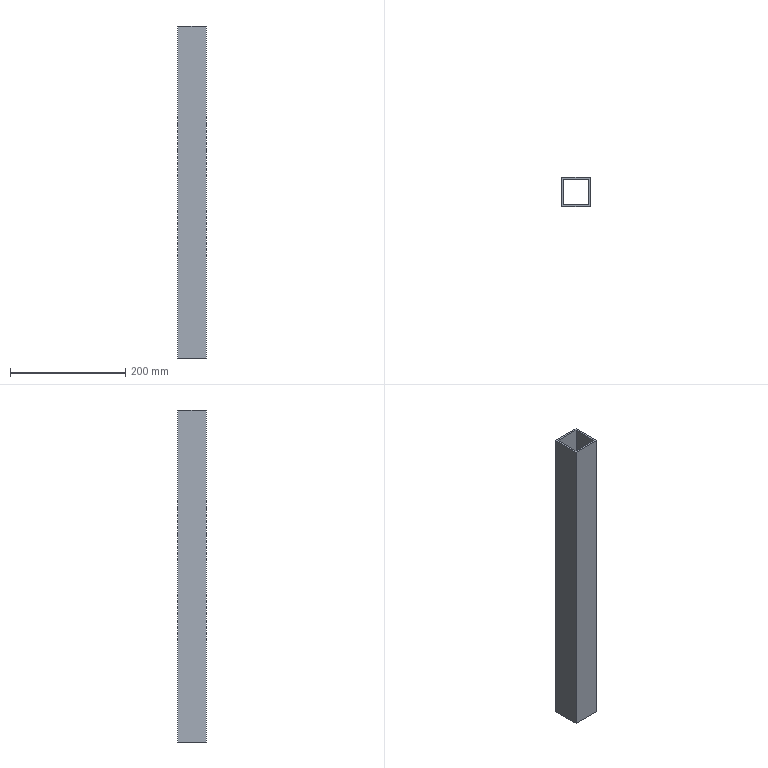Part | SolidWorks | features Cut 1, Extrusion 1 | 1 solid | 10 faces | box 50 x 50 x 575 mm | volume 324300 mm3 | plane 10
STEP:
#1=CARTESIAN_POINT('',(0.,0.,575.));
#2=VERTEX_POINT('',#1);
#3=CARTESIAN_POINT('',(50.,0.,575.));
#4=VERTEX_POINT('',#3);
#5=CARTESIAN_POINT('',(0.,0.,575.));
#6=DIRECTION('',(1.,0.,0.));
#7=VECTOR('',#6,1000.);
#8=LINE('',#5,#7);
#9=EDGE_CURVE('',#2,#4,#8,.T.);
#10=ORIENTED_EDGE('',*,*,#9,.F.);
#11=CARTESIAN_POINT('',(0.,0.,0.));
#12=VERTEX_POINT('',#11);
#13=CARTESIAN_POINT('',(0.,0.,600.));
#14=DIRECTION('',(0.,0.,-1.));
#15=VECTOR('',#14,1000.);
#16=LINE('',#13,#15);
#17=EDGE_CURVE('',#2,#12,#16,.T.);
#18=ORIENTED_EDGE('',*,*,#17,.T.);
#19=CARTESIAN_POINT('',(50.,0.,0.));
#20=VERTEX_POINT('',#19);
#21=CARTESIAN_POINT('',(50.,0.,0.));
#22=DIRECTION('',(1.,0.,0.));
#23=VECTOR('',#22,1000.);
#24=LINE('',#21,#23);
#25=EDGE_CURVE('',#12,#20,#24,.T.);
#26=ORIENTED_EDGE('',*,*,#25,.T.);
#27=CARTESIAN_POINT('',(50.,0.,600.));
#28=DIRECTION('',(0.,0.,-1.));
#29=VECTOR('',#28,1000.);
#30=LINE('',#27,#29);
#31=EDGE_CURVE('',#4,#20,#30,.T.);
#32=ORIENTED_EDGE('',*,*,#31,.F.);
#33=EDGE_LOOP('',(#10,#18,#26,#32));
#34=FACE_OUTER_BOUND('',#33,.T.);
#35=CARTESIAN_POINT('',(50.,0.,600.));
#36=DIRECTION('',(0.,1.,0.));
#37=DIRECTION('',(0.,0.,1.));
#38=AXIS2_PLACEMENT_3D('',#35,#36,#37);
#39=PLANE('',#38);
#40=ADVANCED_FACE('',(#34),#39,.F.);
#41=CARTESIAN_POINT('',(50.,50.,575.));
#42=VERTEX_POINT('',#41);
#43=CARTESIAN_POINT('',(50.,0.,575.));
#44=DIRECTION('',(0.,1.,0.));
#45=VECTOR('',#44,1000.);
#46=LINE('',#43,#45);
#47=EDGE_CURVE('',#4,#42,#46,.T.);
#48=ORIENTED_EDGE('',*,*,#47,.F.);
#49=ORIENTED_EDGE('',*,*,#31,.T.);
#50=CARTESIAN_POINT('',(50.,50.,0.));
#51=VERTEX_POINT('',#50);
#52=CARTESIAN_POINT('',(50.,50.,0.));
#53=DIRECTION('',(0.,1.,0.));
#54=VECTOR('',#53,1000.);
#55=LINE('',#52,#54);
#56=EDGE_CURVE('',#20,#51,#55,.T.);
#57=ORIENTED_EDGE('',*,*,#56,.T.);
#58=CARTESIAN_POINT('',(50.,50.,600.));
#59=DIRECTION('',(0.,0.,-1.));
#60=VECTOR('',#59,1000.);
#61=LINE('',#58,#60);
#62=EDGE_CURVE('',#42,#51,#61,.T.);
#63=ORIENTED_EDGE('',*,*,#62,.F.);
#64=EDGE_LOOP('',(#48,#49,#57,#63));
#65=FACE_OUTER_BOUND('',#64,.T.);
#66=CARTESIAN_POINT('',(50.,50.,600.));
#67=DIRECTION('',(-1.,0.,0.));
#68=DIRECTION('',(0.,0.,1.));
#69=AXIS2_PLACEMENT_3D('',#66,#67,#68);
#70=PLANE('',#69);
#71=ADVANCED_FACE('',(#65),#70,.F.);
#72=CARTESIAN_POINT('',(0.,50.,575.));
#73=VERTEX_POINT('',#72);
#74=CARTESIAN_POINT('',(50.,50.,575.));
#75=DIRECTION('',(-1.,0.,0.));
#76=VECTOR('',#75,1000.);
#77=LINE('',#74,#76);
#78=EDGE_CURVE('',#42,#73,#77,.T.);
#79=ORIENTED_EDGE('',*,*,#78,.F.);
#80=ORIENTED_EDGE('',*,*,#62,.T.);
#81=CARTESIAN_POINT('',(0.,50.,0.));
#82=VERTEX_POINT('',#81);
#83=CARTESIAN_POINT('',(0.,50.,0.));
#84=DIRECTION('',(-1.,0.,0.));
#85=VECTOR('',#84,1000.);
#86=LINE('',#83,#85);
#87=EDGE_CURVE('',#51,#82,#86,.T.);
#88=ORIENTED_EDGE('',*,*,#87,.T.);
#89=CARTESIAN_POINT('',(0.,50.,600.));
#90=DIRECTION('',(0.,0.,-1.));
#91=VECTOR('',#90,1000.);
#92=LINE('',#89,#91);
#93=EDGE_CURVE('',#73,#82,#92,.T.);
#94=ORIENTED_EDGE('',*,*,#93,.F.);
#95=EDGE_LOOP('',(#79,#80,#88,#94));
#96=FACE_OUTER_BOUND('',#95,.T.);
#97=CARTESIAN_POINT('',(0.,50.,600.));
#98=DIRECTION('',(0.,-1.,0.));
#99=DIRECTION('',(0.,0.,-1.));
#100=AXIS2_PLACEMENT_3D('',#97,#98,#99);
#101=PLANE('',#100);
#102=ADVANCED_FACE('',(#96),#101,.F.);
#103=CARTESIAN_POINT('',(0.,50.,575.));
#104=DIRECTION('',(0.,-1.,0.));
#105=VECTOR('',#104,1000.);
#106=LINE('',#103,#105);
#107=EDGE_CURVE('',#73,#2,#106,.T.);
#108=ORIENTED_EDGE('',*,*,#107,.F.);
#109=ORIENTED_EDGE('',*,*,#93,.T.);
#110=CARTESIAN_POINT('',(0.,0.,0.));
#111=DIRECTION('',(0.,-1.,0.));
#112=VECTOR('',#111,1000.);
#113=LINE('',#110,#112);
#114=EDGE_CURVE('',#82,#12,#113,.T.);
#115=ORIENTED_EDGE('',*,*,#114,.T.);
#116=ORIENTED_EDGE('',*,*,#17,.F.);
#117=EDGE_LOOP('',(#108,#109,#115,#116));
#118=FACE_OUTER_BOUND('',#117,.T.);
#119=CARTESIAN_POINT('',(0.,0.,600.));
#120=DIRECTION('',(1.,0.,0.));
#121=DIRECTION('',(0.,0.,-1.));
#122=AXIS2_PLACEMENT_3D('',#119,#120,#121);
#123=PLANE('',#122);
#124=ADVANCED_FACE('',(#118),#123,.F.);
#125=CARTESIAN_POINT('',(3.,3.,575.));
#126=VERTEX_POINT('',#125);
#127=CARTESIAN_POINT('',(3.,3.,0.));
#128=VERTEX_POINT('',#127);
#129=CARTESIAN_POINT('',(3.,3.,600.));
#130=DIRECTION('',(0.,0.,-1.));
#131=VECTOR('',#130,1000.);
#132=LINE('',#129,#131);
#133=EDGE_CURVE('',#126,#128,#132,.T.);
#134=ORIENTED_EDGE('',*,*,#133,.F.);
#135=CARTESIAN_POINT('',(47.,3.,575.));
#136=VERTEX_POINT('',#135);
#137=CARTESIAN_POINT('',(3.,3.,575.));
#138=DIRECTION('',(1.,0.,0.));
#139=VECTOR('',#138,1000.);
#140=LINE('',#137,#139);
#141=EDGE_CURVE('',#126,#136,#140,.T.);
#142=ORIENTED_EDGE('',*,*,#141,.T.);
#143=CARTESIAN_POINT('',(47.,3.,0.));
#144=VERTEX_POINT('',#143);
#145=CARTESIAN_POINT('',(47.,3.,600.));
#146=DIRECTION('',(0.,0.,-1.));
#147=VECTOR('',#146,1000.);
#148=LINE('',#145,#147);
#149=EDGE_CURVE('',#136,#144,#148,.T.);
#150=ORIENTED_EDGE('',*,*,#149,.T.);
#151=CARTESIAN_POINT('',(47.,3.,0.));
#152=DIRECTION('',(1.,0.,0.));
#153=VECTOR('',#152,1000.);
#154=LINE('',#151,#153);
#155=EDGE_CURVE('',#128,#144,#154,.T.);
#156=ORIENTED_EDGE('',*,*,#155,.F.);
#157=EDGE_LOOP('',(#134,#142,#150,#156));
#158=FACE_OUTER_BOUND('',#157,.T.);
#159=CARTESIAN_POINT('',(47.,3.,600.));
#160=DIRECTION('',(0.,1.,0.));
#161=DIRECTION('',(0.,0.,1.));
#162=AXIS2_PLACEMENT_3D('',#159,#160,#161);
#163=PLANE('',#162);
#164=ADVANCED_FACE('',(#158),#163,.T.);
#165=ORIENTED_EDGE('',*,*,#149,.F.);
#166=CARTESIAN_POINT('',(47.,47.,575.));
#167=VERTEX_POINT('',#166);
#168=CARTESIAN_POINT('',(47.,3.,575.));
#169=DIRECTION('',(0.,1.,0.));
#170=VECTOR('',#169,1000.);
#171=LINE('',#168,#170);
#172=EDGE_CURVE('',#136,#167,#171,.T.);
#173=ORIENTED_EDGE('',*,*,#172,.T.);
#174=CARTESIAN_POINT('',(47.,47.,0.));
#175=VERTEX_POINT('',#174);
#176=CARTESIAN_POINT('',(47.,47.,600.));
#177=DIRECTION('',(0.,0.,-1.));
#178=VECTOR('',#177,1000.);
#179=LINE('',#176,#178);
#180=EDGE_CURVE('',#167,#175,#179,.T.);
#181=ORIENTED_EDGE('',*,*,#180,.T.);
#182=CARTESIAN_POINT('',(47.,47.,0.));
#183=DIRECTION('',(0.,1.,0.));
#184=VECTOR('',#183,1000.);
#185=LINE('',#182,#184);
#186=EDGE_CURVE('',#144,#175,#185,.T.);
#187=ORIENTED_EDGE('',*,*,#186,.F.);
#188=EDGE_LOOP('',(#165,#173,#181,#187));
#189=FACE_OUTER_BOUND('',#188,.T.);
#190=CARTESIAN_POINT('',(47.,47.,600.));
#191=DIRECTION('',(-1.,0.,0.));
#192=DIRECTION('',(0.,0.,1.));
#193=AXIS2_PLACEMENT_3D('',#190,#191,#192);
#194=PLANE('',#193);
#195=ADVANCED_FACE('',(#189),#194,.T.);
#196=ORIENTED_EDGE('',*,*,#180,.F.);
#197=CARTESIAN_POINT('',(3.,47.,575.));
#198=VERTEX_POINT('',#197);
#199=CARTESIAN_POINT('',(47.,47.,575.));
#200=DIRECTION('',(-1.,0.,0.));
#201=VECTOR('',#200,1000.);
#202=LINE('',#199,#201);
#203=EDGE_CURVE('',#167,#198,#202,.T.);
#204=ORIENTED_EDGE('',*,*,#203,.T.);
#205=CARTESIAN_POINT('',(3.,47.,0.));
#206=VERTEX_POINT('',#205);
#207=CARTESIAN_POINT('',(3.,47.,600.));
#208=DIRECTION('',(0.,0.,-1.));
#209=VECTOR('',#208,1000.);
#210=LINE('',#207,#209);
#211=EDGE_CURVE('',#198,#206,#210,.T.);
#212=ORIENTED_EDGE('',*,*,#211,.T.);
#213=CARTESIAN_POINT('',(3.,47.,0.));
#214=DIRECTION('',(-1.,0.,0.));
#215=VECTOR('',#214,1000.);
#216=LINE('',#213,#215);
#217=EDGE_CURVE('',#175,#206,#216,.T.);
#218=ORIENTED_EDGE('',*,*,#217,.F.);
#219=EDGE_LOOP('',(#196,#204,#212,#218));
#220=FACE_OUTER_BOUND('',#219,.T.);
#221=CARTESIAN_POINT('',(3.,47.,600.));
#222=DIRECTION('',(0.,-1.,0.));
#223=DIRECTION('',(0.,0.,-1.));
#224=AXIS2_PLACEMENT_3D('',#221,#222,#223);
#225=PLANE('',#224);
#226=ADVANCED_FACE('',(#220),#225,.T.);
#227=ORIENTED_EDGE('',*,*,#211,.F.);
#228=CARTESIAN_POINT('',(3.,47.,575.));
#229=DIRECTION('',(0.,-1.,0.));
#230=VECTOR('',#229,1000.);
#231=LINE('',#228,#230);
#232=EDGE_CURVE('',#198,#126,#231,.T.);
#233=ORIENTED_EDGE('',*,*,#232,.T.);
#234=ORIENTED_EDGE('',*,*,#133,.T.);
#235=CARTESIAN_POINT('',(3.,3.,0.));
#236=DIRECTION('',(0.,-1.,0.));
#237=VECTOR('',#236,1000.);
#238=LINE('',#235,#237);
#239=EDGE_CURVE('',#206,#128,#238,.T.);
#240=ORIENTED_EDGE('',*,*,#239,.F.);
#241=EDGE_LOOP('',(#227,#233,#234,#240));
#242=FACE_OUTER_BOUND('',#241,.T.);
#243=CARTESIAN_POINT('',(3.,3.,600.));
#244=DIRECTION('',(1.,0.,0.));
#245=DIRECTION('',(0.,0.,-1.));
#246=AXIS2_PLACEMENT_3D('',#243,#244,#245);
#247=PLANE('',#246);
#248=ADVANCED_FACE('',(#242),#247,.T.);
#249=ORIENTED_EDGE('',*,*,#25,.F.);
#250=ORIENTED_EDGE('',*,*,#114,.F.);
#251=ORIENTED_EDGE('',*,*,#87,.F.);
#252=ORIENTED_EDGE('',*,*,#56,.F.);
#253=EDGE_LOOP('',(#249,#250,#251,#252));
#254=FACE_OUTER_BOUND('',#253,.T.);
#255=ORIENTED_EDGE('',*,*,#239,.T.);
#256=ORIENTED_EDGE('',*,*,#155,.T.);
#257=ORIENTED_EDGE('',*,*,#186,.T.);
#258=ORIENTED_EDGE('',*,*,#217,.T.);
#259=EDGE_LOOP('',(#255,#256,#257,#258));
#260=FACE_BOUND('',#259,.T.);
#261=CARTESIAN_POINT('',(0.,0.,0.));
#262=DIRECTION('',(0.,0.,-1.));
#263=DIRECTION('',(-1.,0.,0.));
#264=AXIS2_PLACEMENT_3D('',#261,#262,#263);
#265=PLANE('',#264);
#266=ADVANCED_FACE('',(#254,#260),#265,.T.);
#267=ORIENTED_EDGE('',*,*,#232,.F.);
#268=ORIENTED_EDGE('',*,*,#203,.F.);
#269=ORIENTED_EDGE('',*,*,#172,.F.);
#270=ORIENTED_EDGE('',*,*,#141,.F.);
#271=EDGE_LOOP('',(#267,#268,#269,#270));
#272=FACE_BOUND('',#271,.T.);
#273=ORIENTED_EDGE('',*,*,#107,.T.);
#274=ORIENTED_EDGE('',*,*,#9,.T.);
#275=ORIENTED_EDGE('',*,*,#47,.T.);
#276=ORIENTED_EDGE('',*,*,#78,.T.);
#277=EDGE_LOOP('',(#273,#274,#275,#276));
#278=FACE_OUTER_BOUND('',#277,.T.);
#279=CARTESIAN_POINT('',(0.,0.,575.));
#280=DIRECTION('',(0.,0.,1.));
#281=DIRECTION('',(1.,0.,0.));
#282=AXIS2_PLACEMENT_3D('',#279,#280,#281);
#283=PLANE('',#282);
#284=ADVANCED_FACE('',(#272,#278),#283,.T.);
#285=CLOSED_SHELL('',(#40,#71,#102,#124,#164,#195,#226,#248,#266,#284));
#286=MANIFOLD_SOLID_BREP('',#285);
#287=CARTESIAN_POINT('',(0.,0.,0.));
#288=DIRECTION('',(0.,0.,1.));
#289=DIRECTION('',(1.,0.,0.));
#290=AXIS2_PLACEMENT_3D('',#287,#288,#289);
#291=(LENGTH_UNIT()NAMED_UNIT(*)SI_UNIT(.MILLI.,.METRE.));
#292=UNCERTAINTY_MEASURE_WITH_UNIT(LENGTH_MEASURE(0.00001),#291,'','');
#293=(NAMED_UNIT(*)PLANE_ANGLE_UNIT()SI_UNIT($,.RADIAN.));
#294=(NAMED_UNIT(*)SI_UNIT($,.STERADIAN.)SOLID_ANGLE_UNIT());
#295=(GEOMETRIC_REPRESENTATION_CONTEXT(3)GLOBAL_UNCERTAINTY_ASSIGNED_CONTEXT((#292))GLOBAL_UNIT_ASSIGNED_CONTEXT((#291,#293,#294))REPRESENTATION_CONTEXT('',''));
#296=ADVANCED_BREP_SHAPE_REPRESENTATION('',(#286,#290),#295);